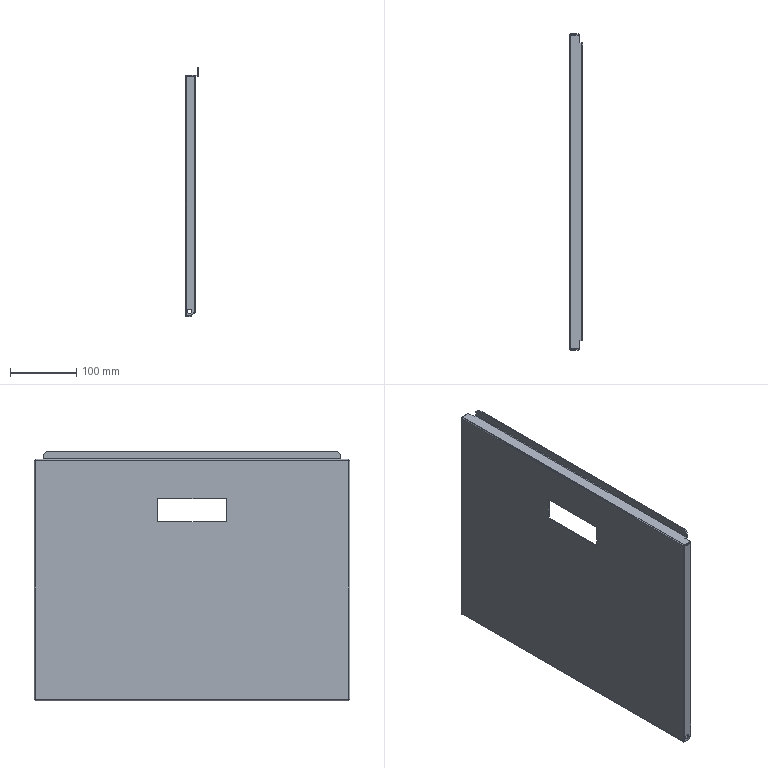Part | SolidWorks | features EdgeFlange 6, ICE 5, Chamfer 1, FlatPattern 1, SMBaseFlange 1, SheetMetal 1 | 1 solid | 96 faces | box 20.237 x 477 x 376.5 mm | volume 311097 mm3 | plane 76 | cylinder 20 | commonest cylinder face diameters 0.6 x6 3.6 x6 7 x4 1.473 x2 4.473 x2